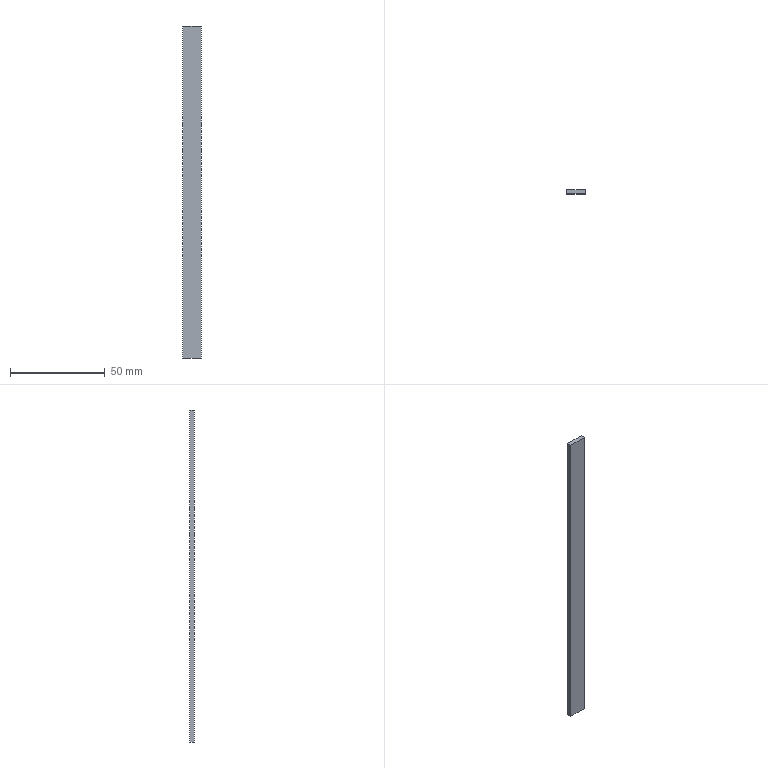Part | SolidWorks | features FlatPattern 1, SMBaseFlange 1, SheetMetal 1 | 1 solid | 6 faces | box 10 x 2.3 x 175 mm | volume 4025 mm3 | plane 6
STEP:
#1=CARTESIAN_POINT('',(5.,0.,87.5));
#2=VERTEX_POINT('',#1);
#3=CARTESIAN_POINT('',(5.,0.,-87.5));
#4=VERTEX_POINT('',#3);
#5=CARTESIAN_POINT('',(5.,0.,-87.5));
#6=DIRECTION('',(0.,0.,-1.));
#7=VECTOR('',#6,1000.);
#8=LINE('',#5,#7);
#9=EDGE_CURVE('',#2,#4,#8,.T.);
#10=ORIENTED_EDGE('',*,*,#9,.F.);
#11=CARTESIAN_POINT('',(5.,-2.3,87.5));
#12=VERTEX_POINT('',#11);
#13=CARTESIAN_POINT('',(5.,-2.3,87.5));
#14=DIRECTION('',(0.,1.,0.));
#15=VECTOR('',#14,1000.);
#16=LINE('',#13,#15);
#17=EDGE_CURVE('',#12,#2,#16,.T.);
#18=ORIENTED_EDGE('',*,*,#17,.F.);
#19=CARTESIAN_POINT('',(5.,-2.3,-87.5));
#20=VERTEX_POINT('',#19);
#21=CARTESIAN_POINT('',(5.,-2.3,-87.5));
#22=DIRECTION('',(0.,0.,-1.));
#23=VECTOR('',#22,1000.);
#24=LINE('',#21,#23);
#25=EDGE_CURVE('',#12,#20,#24,.T.);
#26=ORIENTED_EDGE('',*,*,#25,.T.);
#27=CARTESIAN_POINT('',(5.,-2.3,-87.5));
#28=DIRECTION('',(0.,1.,0.));
#29=VECTOR('',#28,1000.);
#30=LINE('',#27,#29);
#31=EDGE_CURVE('',#20,#4,#30,.T.);
#32=ORIENTED_EDGE('',*,*,#31,.T.);
#33=EDGE_LOOP('',(#10,#18,#26,#32));
#34=FACE_OUTER_BOUND('',#33,.T.);
#35=CARTESIAN_POINT('',(5.,-2.3,-87.5));
#36=DIRECTION('',(1.,0.,0.));
#37=DIRECTION('',(0.,0.,-1.));
#38=AXIS2_PLACEMENT_3D('',#35,#36,#37);
#39=PLANE('',#38);
#40=ADVANCED_FACE('',(#34),#39,.T.);
#41=CARTESIAN_POINT('',(-5.,0.,87.5));
#42=VERTEX_POINT('',#41);
#43=CARTESIAN_POINT('',(-5.,0.,87.5));
#44=DIRECTION('',(1.,0.,0.));
#45=VECTOR('',#44,1000.);
#46=LINE('',#43,#45);
#47=EDGE_CURVE('',#42,#2,#46,.T.);
#48=ORIENTED_EDGE('',*,*,#47,.F.);
#49=CARTESIAN_POINT('',(-5.,-2.3,87.5));
#50=VERTEX_POINT('',#49);
#51=CARTESIAN_POINT('',(-5.,-2.3,87.5));
#52=DIRECTION('',(0.,1.,0.));
#53=VECTOR('',#52,1000.);
#54=LINE('',#51,#53);
#55=EDGE_CURVE('',#50,#42,#54,.T.);
#56=ORIENTED_EDGE('',*,*,#55,.F.);
#57=CARTESIAN_POINT('',(-5.,-2.3,87.5));
#58=DIRECTION('',(1.,0.,0.));
#59=VECTOR('',#58,1000.);
#60=LINE('',#57,#59);
#61=EDGE_CURVE('',#50,#12,#60,.T.);
#62=ORIENTED_EDGE('',*,*,#61,.T.);
#63=ORIENTED_EDGE('',*,*,#17,.T.);
#64=EDGE_LOOP('',(#48,#56,#62,#63));
#65=FACE_OUTER_BOUND('',#64,.T.);
#66=CARTESIAN_POINT('',(-5.,-2.3,87.5));
#67=DIRECTION('',(0.,0.,1.));
#68=DIRECTION('',(1.,0.,0.));
#69=AXIS2_PLACEMENT_3D('',#66,#67,#68);
#70=PLANE('',#69);
#71=ADVANCED_FACE('',(#65),#70,.T.);
#72=CARTESIAN_POINT('',(-5.,0.,-87.5));
#73=VERTEX_POINT('',#72);
#74=CARTESIAN_POINT('',(-5.,0.,-87.5));
#75=DIRECTION('',(0.,0.,1.));
#76=VECTOR('',#75,1000.);
#77=LINE('',#74,#76);
#78=EDGE_CURVE('',#73,#42,#77,.T.);
#79=ORIENTED_EDGE('',*,*,#78,.F.);
#80=CARTESIAN_POINT('',(-5.,-2.3,-87.5));
#81=VERTEX_POINT('',#80);
#82=CARTESIAN_POINT('',(-5.,-2.3,-87.5));
#83=DIRECTION('',(0.,1.,0.));
#84=VECTOR('',#83,1000.);
#85=LINE('',#82,#84);
#86=EDGE_CURVE('',#81,#73,#85,.T.);
#87=ORIENTED_EDGE('',*,*,#86,.F.);
#88=CARTESIAN_POINT('',(-5.,-2.3,-87.5));
#89=DIRECTION('',(0.,0.,1.));
#90=VECTOR('',#89,1000.);
#91=LINE('',#88,#90);
#92=EDGE_CURVE('',#81,#50,#91,.T.);
#93=ORIENTED_EDGE('',*,*,#92,.T.);
#94=ORIENTED_EDGE('',*,*,#55,.T.);
#95=EDGE_LOOP('',(#79,#87,#93,#94));
#96=FACE_OUTER_BOUND('',#95,.T.);
#97=CARTESIAN_POINT('',(-5.,-2.3,-87.5));
#98=DIRECTION('',(-1.,0.,0.));
#99=DIRECTION('',(0.,0.,1.));
#100=AXIS2_PLACEMENT_3D('',#97,#98,#99);
#101=PLANE('',#100);
#102=ADVANCED_FACE('',(#96),#101,.T.);
#103=CARTESIAN_POINT('',(-5.,0.,-87.5));
#104=DIRECTION('',(-1.,0.,0.));
#105=VECTOR('',#104,1000.);
#106=LINE('',#103,#105);
#107=EDGE_CURVE('',#4,#73,#106,.T.);
#108=ORIENTED_EDGE('',*,*,#107,.F.);
#109=ORIENTED_EDGE('',*,*,#31,.F.);
#110=CARTESIAN_POINT('',(-5.,-2.3,-87.5));
#111=DIRECTION('',(-1.,0.,0.));
#112=VECTOR('',#111,1000.);
#113=LINE('',#110,#112);
#114=EDGE_CURVE('',#20,#81,#113,.T.);
#115=ORIENTED_EDGE('',*,*,#114,.T.);
#116=ORIENTED_EDGE('',*,*,#86,.T.);
#117=EDGE_LOOP('',(#108,#109,#115,#116));
#118=FACE_OUTER_BOUND('',#117,.T.);
#119=CARTESIAN_POINT('',(-5.,-2.3,-87.5));
#120=DIRECTION('',(0.,0.,-1.));
#121=DIRECTION('',(-1.,0.,0.));
#122=AXIS2_PLACEMENT_3D('',#119,#120,#121);
#123=PLANE('',#122);
#124=ADVANCED_FACE('',(#118),#123,.T.);
#125=ORIENTED_EDGE('',*,*,#25,.F.);
#126=ORIENTED_EDGE('',*,*,#61,.F.);
#127=ORIENTED_EDGE('',*,*,#92,.F.);
#128=ORIENTED_EDGE('',*,*,#114,.F.);
#129=EDGE_LOOP('',(#125,#126,#127,#128));
#130=FACE_OUTER_BOUND('',#129,.T.);
#131=CARTESIAN_POINT('',(0.,-2.3,0.));
#132=DIRECTION('',(0.,1.,0.));
#133=DIRECTION('',(0.,0.,1.));
#134=AXIS2_PLACEMENT_3D('',#131,#132,#133);
#135=PLANE('',#134);
#136=ADVANCED_FACE('',(#130),#135,.F.);
#137=ORIENTED_EDGE('',*,*,#9,.T.);
#138=ORIENTED_EDGE('',*,*,#107,.T.);
#139=ORIENTED_EDGE('',*,*,#78,.T.);
#140=ORIENTED_EDGE('',*,*,#47,.T.);
#141=EDGE_LOOP('',(#137,#138,#139,#140));
#142=FACE_OUTER_BOUND('',#141,.T.);
#143=CARTESIAN_POINT('',(0.,0.,0.));
#144=DIRECTION('',(0.,1.,0.));
#145=DIRECTION('',(0.,0.,1.));
#146=AXIS2_PLACEMENT_3D('',#143,#144,#145);
#147=PLANE('',#146);
#148=ADVANCED_FACE('',(#142),#147,.T.);
#149=CLOSED_SHELL('',(#40,#71,#102,#124,#136,#148));
#150=MANIFOLD_SOLID_BREP('',#149);
#151=CARTESIAN_POINT('',(0.,0.,0.));
#152=DIRECTION('',(0.,0.,1.));
#153=DIRECTION('',(1.,0.,0.));
#154=AXIS2_PLACEMENT_3D('',#151,#152,#153);
#155=(LENGTH_UNIT()NAMED_UNIT(*)SI_UNIT(.MILLI.,.METRE.));
#156=UNCERTAINTY_MEASURE_WITH_UNIT(LENGTH_MEASURE(0.00001),#155,'','');
#157=(NAMED_UNIT(*)PLANE_ANGLE_UNIT()SI_UNIT($,.RADIAN.));
#158=(NAMED_UNIT(*)SI_UNIT($,.STERADIAN.)SOLID_ANGLE_UNIT());
#159=(GEOMETRIC_REPRESENTATION_CONTEXT(3)GLOBAL_UNCERTAINTY_ASSIGNED_CONTEXT((#156))GLOBAL_UNIT_ASSIGNED_CONTEXT((#155,#157,#158))REPRESENTATION_CONTEXT('',''));
#160=ADVANCED_BREP_SHAPE_REPRESENTATION('',(#150,#154),#159);